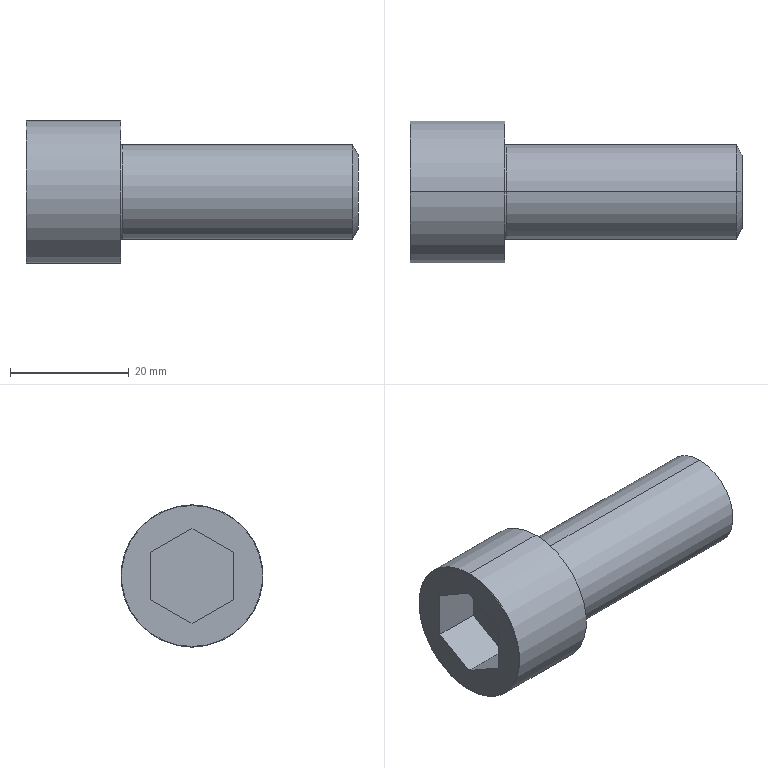Part | SolidWorks | features BlendCut 1, Cut 1, Fillet 1, LPattern 1, RevCut 1, Revolution 1 | 1 solid | 20 faces | box 56 x 24 x 24 mm | volume 13910 mm3 | plane 10 | torus 4 | cylinder 4 | cone 2 | commonest cylinder face diameters 16 x2 24 x2
STEP:
#1=CARTESIAN_POINT('',(0.,0.,11.9));
#2=VERTEX_POINT('',#1);
#3=CARTESIAN_POINT('',(0.,0.,-11.9));
#4=VERTEX_POINT('',#3);
#5=CARTESIAN_POINT('',(0.,0.,0.));
#6=DIRECTION('',(-1.,0.,0.));
#7=DIRECTION('',(0.,0.,-1.));
#8=AXIS2_PLACEMENT_3D('',#5,#6,#7);
#9=CIRCLE('',#8,11.9);
#10=EDGE_CURVE('',#2,#4,#9,.T.);
#11=ORIENTED_EDGE('',*,*,#10,.F.);
#12=CARTESIAN_POINT('',(0.1,0.,12.));
#13=VERTEX_POINT('',#12);
#14=CARTESIAN_POINT('',(0.1,0.,11.9));
#15=DIRECTION('',(0.,1.,0.));
#16=DIRECTION('',(0.,0.,1.));
#17=AXIS2_PLACEMENT_3D('',#14,#15,#16);
#18=CIRCLE('',#17,0.1);
#19=EDGE_CURVE('',#2,#13,#18,.T.);
#20=ORIENTED_EDGE('',*,*,#19,.T.);
#21=CARTESIAN_POINT('',(0.1,0.,-12.));
#22=VERTEX_POINT('',#21);
#23=CARTESIAN_POINT('',(0.1,0.,0.));
#24=DIRECTION('',(1.,0.,0.));
#25=DIRECTION('',(0.,0.,-1.));
#26=AXIS2_PLACEMENT_3D('',#23,#24,#25);
#27=CIRCLE('',#26,12.);
#28=EDGE_CURVE('',#22,#13,#27,.T.);
#29=ORIENTED_EDGE('',*,*,#28,.F.);
#30=CARTESIAN_POINT('',(0.1,0.,-11.9));
#31=DIRECTION('',(0.,-1.,0.));
#32=DIRECTION('',(0.,0.,-1.));
#33=AXIS2_PLACEMENT_3D('',#30,#31,#32);
#34=CIRCLE('',#33,0.1);
#35=EDGE_CURVE('',#4,#22,#34,.T.);
#36=ORIENTED_EDGE('',*,*,#35,.F.);
#37=EDGE_LOOP('',(#11,#20,#29,#36));
#38=FACE_OUTER_BOUND('',#37,.T.);
#39=CARTESIAN_POINT('',(0.1,0.,0.));
#40=DIRECTION('',(1.,0.,0.));
#41=DIRECTION('',(0.,0.,-1.));
#42=AXIS2_PLACEMENT_3D('',#39,#40,#41);
#43=TOROIDAL_SURFACE('',#42,11.9,0.1);
#44=ADVANCED_FACE('',(#38),#43,.T.);
#45=CARTESIAN_POINT('',(56.,0.,6.268));
#46=VERTEX_POINT('',#45);
#47=CARTESIAN_POINT('',(56.,0.,-6.268));
#48=VERTEX_POINT('',#47);
#49=CARTESIAN_POINT('',(56.,0.,0.));
#50=DIRECTION('',(-1.,0.,0.));
#51=DIRECTION('',(0.,0.,1.));
#52=AXIS2_PLACEMENT_3D('',#49,#50,#51);
#53=CIRCLE('',#52,6.268);
#54=EDGE_CURVE('',#46,#48,#53,.T.);
#55=ORIENTED_EDGE('',*,*,#54,.T.);
#56=CARTESIAN_POINT('',(55.,0.,-8.));
#57=VERTEX_POINT('',#56);
#58=CARTESIAN_POINT('',(55.,0.,-8.));
#59=DIRECTION('',(-0.5,0.,-0.866));
#60=VECTOR('',#59,1000.);
#61=LINE('',#58,#60);
#62=EDGE_CURVE('',#48,#57,#61,.T.);
#63=ORIENTED_EDGE('',*,*,#62,.T.);
#64=CARTESIAN_POINT('',(55.,0.,8.));
#65=VERTEX_POINT('',#64);
#66=CARTESIAN_POINT('',(55.,0.,0.));
#67=DIRECTION('',(-1.,0.,0.));
#68=DIRECTION('',(0.,0.,1.));
#69=AXIS2_PLACEMENT_3D('',#66,#67,#68);
#70=CIRCLE('',#69,8.);
#71=EDGE_CURVE('',#65,#57,#70,.T.);
#72=ORIENTED_EDGE('',*,*,#71,.F.);
#73=CARTESIAN_POINT('',(55.,0.,8.));
#74=DIRECTION('',(-0.5,0.,0.866));
#75=VECTOR('',#74,1000.);
#76=LINE('',#73,#75);
#77=EDGE_CURVE('',#46,#65,#76,.T.);
#78=ORIENTED_EDGE('',*,*,#77,.F.);
#79=EDGE_LOOP('',(#55,#63,#72,#78));
#80=FACE_OUTER_BOUND('',#79,.T.);
#81=CARTESIAN_POINT('',(55.,0.,0.));
#82=DIRECTION('',(-1.,0.,0.));
#83=DIRECTION('',(0.,0.,1.));
#84=AXIS2_PLACEMENT_3D('',#81,#82,#83);
#85=CONICAL_SURFACE('',#84,8.,1.047);
#86=ADVANCED_FACE('',(#80),#85,.T.);
#87=CARTESIAN_POINT('',(16.,0.,-8.2));
#88=VERTEX_POINT('',#87);
#89=CARTESIAN_POINT('',(16.,0.,8.2));
#90=VERTEX_POINT('',#89);
#91=CARTESIAN_POINT('',(16.,0.,0.));
#92=DIRECTION('',(-1.,0.,0.));
#93=DIRECTION('',(0.,0.,1.));
#94=AXIS2_PLACEMENT_3D('',#91,#92,#93);
#95=CIRCLE('',#94,8.2);
#96=EDGE_CURVE('',#88,#90,#95,.T.);
#97=ORIENTED_EDGE('',*,*,#96,.F.);
#98=CARTESIAN_POINT('',(16.2,0.,-8.));
#99=VERTEX_POINT('',#98);
#100=CARTESIAN_POINT('',(16.2,0.,-8.2));
#101=DIRECTION('',(0.,1.,0.));
#102=DIRECTION('',(0.,0.,1.));
#103=AXIS2_PLACEMENT_3D('',#100,#101,#102);
#104=CIRCLE('',#103,0.2);
#105=EDGE_CURVE('',#88,#99,#104,.T.);
#106=ORIENTED_EDGE('',*,*,#105,.T.);
#107=CARTESIAN_POINT('',(16.2,0.,8.));
#108=VERTEX_POINT('',#107);
#109=CARTESIAN_POINT('',(16.2,0.,0.));
#110=DIRECTION('',(-1.,0.,0.));
#111=DIRECTION('',(0.,0.,1.));
#112=AXIS2_PLACEMENT_3D('',#109,#110,#111);
#113=CIRCLE('',#112,8.);
#114=EDGE_CURVE('',#99,#108,#113,.T.);
#115=ORIENTED_EDGE('',*,*,#114,.T.);
#116=CARTESIAN_POINT('',(16.2,0.,8.2));
#117=DIRECTION('',(0.,-1.,0.));
#118=DIRECTION('',(0.,0.,-1.));
#119=AXIS2_PLACEMENT_3D('',#116,#117,#118);
#120=CIRCLE('',#119,0.2);
#121=EDGE_CURVE('',#90,#108,#120,.T.);
#122=ORIENTED_EDGE('',*,*,#121,.F.);
#123=EDGE_LOOP('',(#97,#106,#115,#122));
#124=FACE_OUTER_BOUND('',#123,.T.);
#125=CARTESIAN_POINT('',(16.2,0.,0.));
#126=DIRECTION('',(-1.,0.,0.));
#127=DIRECTION('',(0.,0.,1.));
#128=AXIS2_PLACEMENT_3D('',#125,#126,#127);
#129=TOROIDAL_SURFACE('',#128,8.2,0.2);
#130=ADVANCED_FACE('',(#124),#129,.F.);
#131=CARTESIAN_POINT('',(16.,0.,12.));
#132=VERTEX_POINT('',#131);
#133=CARTESIAN_POINT('',(16.,0.,-12.));
#134=VERTEX_POINT('',#133);
#135=CARTESIAN_POINT('',(16.,0.,0.));
#136=DIRECTION('',(-1.,0.,0.));
#137=DIRECTION('',(0.,0.,1.));
#138=AXIS2_PLACEMENT_3D('',#135,#136,#137);
#139=CIRCLE('',#138,12.);
#140=EDGE_CURVE('',#132,#134,#139,.T.);
#141=ORIENTED_EDGE('',*,*,#140,.T.);
#142=CARTESIAN_POINT('',(0.,0.,-12.));
#143=DIRECTION('',(-1.,0.,0.));
#144=VECTOR('',#143,1000.);
#145=LINE('',#142,#144);
#146=EDGE_CURVE('',#134,#22,#145,.T.);
#147=ORIENTED_EDGE('',*,*,#146,.T.);
#148=ORIENTED_EDGE('',*,*,#28,.T.);
#149=CARTESIAN_POINT('',(0.,0.,12.));
#150=DIRECTION('',(-1.,0.,0.));
#151=VECTOR('',#150,1000.);
#152=LINE('',#149,#151);
#153=EDGE_CURVE('',#132,#13,#152,.T.);
#154=ORIENTED_EDGE('',*,*,#153,.F.);
#155=EDGE_LOOP('',(#141,#147,#148,#154));
#156=FACE_OUTER_BOUND('',#155,.T.);
#157=CARTESIAN_POINT('',(0.,0.,0.));
#158=DIRECTION('',(-1.,0.,0.));
#159=DIRECTION('',(0.,0.,1.));
#160=AXIS2_PLACEMENT_3D('',#157,#158,#159);
#161=CYLINDRICAL_SURFACE('',#160,12.);
#162=ADVANCED_FACE('',(#156),#161,.T.);
#163=ORIENTED_EDGE('',*,*,#71,.T.);
#164=CARTESIAN_POINT('',(0.,0.,-8.));
#165=DIRECTION('',(-1.,0.,0.));
#166=VECTOR('',#165,1000.);
#167=LINE('',#164,#166);
#168=EDGE_CURVE('',#57,#99,#167,.T.);
#169=ORIENTED_EDGE('',*,*,#168,.T.);
#170=CARTESIAN_POINT('',(16.2,0.,0.));
#171=DIRECTION('',(-1.,0.,0.));
#172=DIRECTION('',(0.,0.,1.));
#173=AXIS2_PLACEMENT_3D('',#170,#171,#172);
#174=CIRCLE('',#173,8.);
#175=EDGE_CURVE('',#108,#99,#174,.T.);
#176=ORIENTED_EDGE('',*,*,#175,.F.);
#177=CARTESIAN_POINT('',(0.,0.,8.));
#178=DIRECTION('',(-1.,0.,0.));
#179=VECTOR('',#178,1000.);
#180=LINE('',#177,#179);
#181=EDGE_CURVE('',#65,#108,#180,.T.);
#182=ORIENTED_EDGE('',*,*,#181,.F.);
#183=EDGE_LOOP('',(#163,#169,#176,#182));
#184=FACE_OUTER_BOUND('',#183,.T.);
#185=CARTESIAN_POINT('',(0.,0.,0.));
#186=DIRECTION('',(-1.,0.,0.));
#187=DIRECTION('',(0.,0.,1.));
#188=AXIS2_PLACEMENT_3D('',#185,#186,#187);
#189=CYLINDRICAL_SURFACE('',#188,8.);
#190=ADVANCED_FACE('',(#184),#189,.T.);
#191=ORIENTED_EDGE('',*,*,#168,.F.);
#192=CARTESIAN_POINT('',(55.,0.,0.));
#193=DIRECTION('',(-1.,0.,0.));
#194=DIRECTION('',(0.,0.,1.));
#195=AXIS2_PLACEMENT_3D('',#192,#193,#194);
#196=CIRCLE('',#195,8.);
#197=EDGE_CURVE('',#57,#65,#196,.T.);
#198=ORIENTED_EDGE('',*,*,#197,.T.);
#199=ORIENTED_EDGE('',*,*,#181,.T.);
#200=ORIENTED_EDGE('',*,*,#114,.F.);
#201=EDGE_LOOP('',(#191,#198,#199,#200));
#202=FACE_OUTER_BOUND('',#201,.T.);
#203=CARTESIAN_POINT('',(0.,0.,0.));
#204=DIRECTION('',(-1.,0.,0.));
#205=DIRECTION('',(0.,0.,1.));
#206=AXIS2_PLACEMENT_3D('',#203,#204,#205);
#207=CYLINDRICAL_SURFACE('',#206,8.);
#208=ADVANCED_FACE('',(#202),#207,.T.);
#209=CARTESIAN_POINT('',(0.,0.,0.));
#210=DIRECTION('',(-1.,0.,0.));
#211=DIRECTION('',(0.,0.,-1.));
#212=AXIS2_PLACEMENT_3D('',#209,#210,#211);
#213=CIRCLE('',#212,11.9);
#214=EDGE_CURVE('',#4,#2,#213,.T.);
#215=ORIENTED_EDGE('',*,*,#214,.T.);
#216=ORIENTED_EDGE('',*,*,#10,.T.);
#217=EDGE_LOOP('',(#215,#216));
#218=FACE_OUTER_BOUND('',#217,.T.);
#219=CARTESIAN_POINT('',(0.,0.,8.));
#220=VERTEX_POINT('',#219);
#221=CARTESIAN_POINT('',(0.,6.928,4.));
#222=VERTEX_POINT('',#221);
#223=CARTESIAN_POINT('',(0.,0.,8.));
#224=DIRECTION('',(0.,0.866,-0.5));
#225=VECTOR('',#224,1000.);
#226=LINE('',#223,#225);
#227=EDGE_CURVE('',#220,#222,#226,.T.);
#228=ORIENTED_EDGE('',*,*,#227,.F.);
#229=CARTESIAN_POINT('',(0.,-6.928,4.));
#230=VERTEX_POINT('',#229);
#231=CARTESIAN_POINT('',(0.,-6.928,4.));
#232=DIRECTION('',(0.,0.866,0.5));
#233=VECTOR('',#232,1000.);
#234=LINE('',#231,#233);
#235=EDGE_CURVE('',#230,#220,#234,.T.);
#236=ORIENTED_EDGE('',*,*,#235,.F.);
#237=CARTESIAN_POINT('',(0.,-6.928,-4.));
#238=VERTEX_POINT('',#237);
#239=CARTESIAN_POINT('',(0.,-6.928,-4.));
#240=DIRECTION('',(0.,0.,1.));
#241=VECTOR('',#240,1000.);
#242=LINE('',#239,#241);
#243=EDGE_CURVE('',#238,#230,#242,.T.);
#244=ORIENTED_EDGE('',*,*,#243,.F.);
#245=CARTESIAN_POINT('',(0.,0.,-8.));
#246=VERTEX_POINT('',#245);
#247=CARTESIAN_POINT('',(0.,0.,-8.));
#248=DIRECTION('',(0.,-0.866,0.5));
#249=VECTOR('',#248,1000.);
#250=LINE('',#247,#249);
#251=EDGE_CURVE('',#246,#238,#250,.T.);
#252=ORIENTED_EDGE('',*,*,#251,.F.);
#253=CARTESIAN_POINT('',(0.,6.928,-4.));
#254=VERTEX_POINT('',#253);
#255=CARTESIAN_POINT('',(0.,6.928,-4.));
#256=DIRECTION('',(0.,-0.866,-0.5));
#257=VECTOR('',#256,1000.);
#258=LINE('',#255,#257);
#259=EDGE_CURVE('',#254,#246,#258,.T.);
#260=ORIENTED_EDGE('',*,*,#259,.F.);
#261=CARTESIAN_POINT('',(0.,6.928,4.));
#262=DIRECTION('',(0.,0.,-1.));
#263=VECTOR('',#262,1000.);
#264=LINE('',#261,#263);
#265=EDGE_CURVE('',#222,#254,#264,.T.);
#266=ORIENTED_EDGE('',*,*,#265,.F.);
#267=EDGE_LOOP('',(#228,#236,#244,#252,#260,#266));
#268=FACE_BOUND('',#267,.T.);
#269=CARTESIAN_POINT('',(0.,0.,0.));
#270=DIRECTION('',(1.,0.,0.));
#271=DIRECTION('',(0.,0.,-1.));
#272=AXIS2_PLACEMENT_3D('',#269,#270,#271);
#273=PLANE('',#272);
#274=ADVANCED_FACE('',(#218,#268),#273,.F.);
#275=ORIENTED_EDGE('',*,*,#146,.F.);
#276=CARTESIAN_POINT('',(16.,0.,0.));
#277=DIRECTION('',(-1.,0.,0.));
#278=DIRECTION('',(0.,0.,1.));
#279=AXIS2_PLACEMENT_3D('',#276,#277,#278);
#280=CIRCLE('',#279,12.);
#281=EDGE_CURVE('',#134,#132,#280,.T.);
#282=ORIENTED_EDGE('',*,*,#281,.T.);
#283=ORIENTED_EDGE('',*,*,#153,.T.);
#284=CARTESIAN_POINT('',(0.1,0.,0.));
#285=DIRECTION('',(1.,0.,0.));
#286=DIRECTION('',(0.,0.,-1.));
#287=AXIS2_PLACEMENT_3D('',#284,#285,#286);
#288=CIRCLE('',#287,12.);
#289=EDGE_CURVE('',#13,#22,#288,.T.);
#290=ORIENTED_EDGE('',*,*,#289,.T.);
#291=EDGE_LOOP('',(#275,#282,#283,#290));
#292=FACE_OUTER_BOUND('',#291,.T.);
#293=CARTESIAN_POINT('',(0.,0.,0.));
#294=DIRECTION('',(-1.,0.,0.));
#295=DIRECTION('',(0.,0.,1.));
#296=AXIS2_PLACEMENT_3D('',#293,#294,#295);
#297=CYLINDRICAL_SURFACE('',#296,12.);
#298=ADVANCED_FACE('',(#292),#297,.T.);
#299=ORIENTED_EDGE('',*,*,#140,.F.);
#300=ORIENTED_EDGE('',*,*,#281,.F.);
#301=EDGE_LOOP('',(#299,#300));
#302=FACE_OUTER_BOUND('',#301,.T.);
#303=CARTESIAN_POINT('',(16.,0.,0.));
#304=DIRECTION('',(-1.,0.,0.));
#305=DIRECTION('',(0.,0.,1.));
#306=AXIS2_PLACEMENT_3D('',#303,#304,#305);
#307=CIRCLE('',#306,8.2);
#308=EDGE_CURVE('',#90,#88,#307,.T.);
#309=ORIENTED_EDGE('',*,*,#308,.T.);
#310=ORIENTED_EDGE('',*,*,#96,.T.);
#311=EDGE_LOOP('',(#309,#310));
#312=FACE_BOUND('',#311,.T.);
#313=CARTESIAN_POINT('',(16.,12.,0.));
#314=DIRECTION('',(-1.,0.,0.));
#315=DIRECTION('',(0.,0.,1.));
#316=AXIS2_PLACEMENT_3D('',#313,#314,#315);
#317=PLANE('',#316);
#318=ADVANCED_FACE('',(#302,#312),#317,.F.);
#319=ORIENTED_EDGE('',*,*,#105,.F.);
#320=ORIENTED_EDGE('',*,*,#308,.F.);
#321=ORIENTED_EDGE('',*,*,#121,.T.);
#322=ORIENTED_EDGE('',*,*,#175,.T.);
#323=EDGE_LOOP('',(#319,#320,#321,#322));
#324=FACE_OUTER_BOUND('',#323,.T.);
#325=CARTESIAN_POINT('',(16.2,0.,0.));
#326=DIRECTION('',(-1.,0.,0.));
#327=DIRECTION('',(0.,0.,1.));
#328=AXIS2_PLACEMENT_3D('',#325,#326,#327);
#329=TOROIDAL_SURFACE('',#328,8.2,0.2);
#330=ADVANCED_FACE('',(#324),#329,.F.);
#331=ORIENTED_EDGE('',*,*,#235,.T.);
#332=CARTESIAN_POINT('',(8.,0.,8.));
#333=VERTEX_POINT('',#332);
#334=CARTESIAN_POINT('',(8.,0.,8.));
#335=DIRECTION('',(-1.,0.,0.));
#336=VECTOR('',#335,1000.);
#337=LINE('',#334,#336);
#338=EDGE_CURVE('',#333,#220,#337,.T.);
#339=ORIENTED_EDGE('',*,*,#338,.F.);
#340=CARTESIAN_POINT('',(8.,-6.928,4.));
#341=VERTEX_POINT('',#340);
#342=CARTESIAN_POINT('',(8.,-6.928,4.));
#343=DIRECTION('',(0.,0.866,0.5));
#344=VECTOR('',#343,1000.);
#345=LINE('',#342,#344);
#346=EDGE_CURVE('',#341,#333,#345,.T.);
#347=ORIENTED_EDGE('',*,*,#346,.F.);
#348=CARTESIAN_POINT('',(8.,-6.928,4.));
#349=DIRECTION('',(-1.,0.,0.));
#350=VECTOR('',#349,1000.);
#351=LINE('',#348,#350);
#352=EDGE_CURVE('',#341,#230,#351,.T.);
#353=ORIENTED_EDGE('',*,*,#352,.T.);
#354=EDGE_LOOP('',(#331,#339,#347,#353));
#355=FACE_OUTER_BOUND('',#354,.T.);
#356=CARTESIAN_POINT('',(8.,-6.928,4.));
#357=DIRECTION('',(0.,-0.5,0.866));
#358=DIRECTION('',(0.,-0.866,-0.5));
#359=AXIS2_PLACEMENT_3D('',#356,#357,#358);
#360=PLANE('',#359);
#361=ADVANCED_FACE('',(#355),#360,.F.);
#362=ORIENTED_EDGE('',*,*,#243,.T.);
#363=ORIENTED_EDGE('',*,*,#352,.F.);
#364=CARTESIAN_POINT('',(8.,-6.928,-4.));
#365=VERTEX_POINT('',#364);
#366=CARTESIAN_POINT('',(8.,-6.928,-4.));
#367=DIRECTION('',(0.,0.,1.));
#368=VECTOR('',#367,1000.);
#369=LINE('',#366,#368);
#370=EDGE_CURVE('',#365,#341,#369,.T.);
#371=ORIENTED_EDGE('',*,*,#370,.F.);
#372=CARTESIAN_POINT('',(8.,-6.928,-4.));
#373=DIRECTION('',(-1.,0.,0.));
#374=VECTOR('',#373,1000.);
#375=LINE('',#372,#374);
#376=EDGE_CURVE('',#365,#238,#375,.T.);
#377=ORIENTED_EDGE('',*,*,#376,.T.);
#378=EDGE_LOOP('',(#362,#363,#371,#377));
#379=FACE_OUTER_BOUND('',#378,.T.);
#380=CARTESIAN_POINT('',(8.,-6.928,-4.));
#381=DIRECTION('',(0.,-1.,0.));
#382=DIRECTION('',(0.,0.,-1.));
#383=AXIS2_PLACEMENT_3D('',#380,#381,#382);
#384=PLANE('',#383);
#385=ADVANCED_FACE('',(#379),#384,.F.);
#386=ORIENTED_EDGE('',*,*,#251,.T.);
#387=ORIENTED_EDGE('',*,*,#376,.F.);
#388=CARTESIAN_POINT('',(8.,0.,-8.));
#389=VERTEX_POINT('',#388);
#390=CARTESIAN_POINT('',(8.,0.,-8.));
#391=DIRECTION('',(0.,-0.866,0.5));
#392=VECTOR('',#391,1000.);
#393=LINE('',#390,#392);
#394=EDGE_CURVE('',#389,#365,#393,.T.);
#395=ORIENTED_EDGE('',*,*,#394,.F.);
#396=CARTESIAN_POINT('',(8.,0.,-8.));
#397=DIRECTION('',(-1.,0.,0.));
#398=VECTOR('',#397,1000.);
#399=LINE('',#396,#398);
#400=EDGE_CURVE('',#389,#246,#399,.T.);
#401=ORIENTED_EDGE('',*,*,#400,.T.);
#402=EDGE_LOOP('',(#386,#387,#395,#401));
#403=FACE_OUTER_BOUND('',#402,.T.);
#404=CARTESIAN_POINT('',(8.,0.,-8.));
#405=DIRECTION('',(0.,-0.5,-0.866));
#406=DIRECTION('',(0.,0.866,-0.5));
#407=AXIS2_PLACEMENT_3D('',#404,#405,#406);
#408=PLANE('',#407);
#409=ADVANCED_FACE('',(#403),#408,.F.);
#410=ORIENTED_EDGE('',*,*,#259,.T.);
#411=ORIENTED_EDGE('',*,*,#400,.F.);
#412=CARTESIAN_POINT('',(8.,6.928,-4.));
#413=VERTEX_POINT('',#412);
#414=CARTESIAN_POINT('',(8.,6.928,-4.));
#415=DIRECTION('',(0.,-0.866,-0.5));
#416=VECTOR('',#415,1000.);
#417=LINE('',#414,#416);
#418=EDGE_CURVE('',#413,#389,#417,.T.);
#419=ORIENTED_EDGE('',*,*,#418,.F.);
#420=CARTESIAN_POINT('',(8.,6.928,-4.));
#421=DIRECTION('',(-1.,0.,0.));
#422=VECTOR('',#421,1000.);
#423=LINE('',#420,#422);
#424=EDGE_CURVE('',#413,#254,#423,.T.);
#425=ORIENTED_EDGE('',*,*,#424,.T.);
#426=EDGE_LOOP('',(#410,#411,#419,#425));
#427=FACE_OUTER_BOUND('',#426,.T.);
#428=CARTESIAN_POINT('',(8.,6.928,-4.));
#429=DIRECTION('',(0.,0.5,-0.866));
#430=DIRECTION('',(0.,0.866,0.5));
#431=AXIS2_PLACEMENT_3D('',#428,#429,#430);
#432=PLANE('',#431);
#433=ADVANCED_FACE('',(#427),#432,.F.);
#434=ORIENTED_EDGE('',*,*,#265,.T.);
#435=ORIENTED_EDGE('',*,*,#424,.F.);
#436=CARTESIAN_POINT('',(8.,6.928,4.));
#437=VERTEX_POINT('',#436);
#438=CARTESIAN_POINT('',(8.,6.928,4.));
#439=DIRECTION('',(0.,0.,-1.));
#440=VECTOR('',#439,1000.);
#441=LINE('',#438,#440);
#442=EDGE_CURVE('',#437,#413,#441,.T.);
#443=ORIENTED_EDGE('',*,*,#442,.F.);
#444=CARTESIAN_POINT('',(8.,6.928,4.));
#445=DIRECTION('',(-1.,0.,0.));
#446=VECTOR('',#445,1000.);
#447=LINE('',#444,#446);
#448=EDGE_CURVE('',#437,#222,#447,.T.);
#449=ORIENTED_EDGE('',*,*,#448,.T.);
#450=EDGE_LOOP('',(#434,#435,#443,#449));
#451=FACE_OUTER_BOUND('',#450,.T.);
#452=CARTESIAN_POINT('',(8.,6.928,4.));
#453=DIRECTION('',(0.,1.,0.));
#454=DIRECTION('',(0.,0.,1.));
#455=AXIS2_PLACEMENT_3D('',#452,#453,#454);
#456=PLANE('',#455);
#457=ADVANCED_FACE('',(#451),#456,.F.);
#458=ORIENTED_EDGE('',*,*,#227,.T.);
#459=ORIENTED_EDGE('',*,*,#448,.F.);
#460=CARTESIAN_POINT('',(8.,0.,8.));
#461=DIRECTION('',(0.,0.866,-0.5));
#462=VECTOR('',#461,1000.);
#463=LINE('',#460,#462);
#464=EDGE_CURVE('',#333,#437,#463,.T.);
#465=ORIENTED_EDGE('',*,*,#464,.F.);
#466=ORIENTED_EDGE('',*,*,#338,.T.);
#467=EDGE_LOOP('',(#458,#459,#465,#466));
#468=FACE_OUTER_BOUND('',#467,.T.);
#469=CARTESIAN_POINT('',(8.,0.,8.));
#470=DIRECTION('',(0.,0.5,0.866));
#471=DIRECTION('',(0.,-0.866,0.5));
#472=AXIS2_PLACEMENT_3D('',#469,#470,#471);
#473=PLANE('',#472);
#474=ADVANCED_FACE('',(#468),#473,.F.);
#475=ORIENTED_EDGE('',*,*,#346,.T.);
#476=ORIENTED_EDGE('',*,*,#464,.T.);
#477=ORIENTED_EDGE('',*,*,#442,.T.);
#478=ORIENTED_EDGE('',*,*,#418,.T.);
#479=ORIENTED_EDGE('',*,*,#394,.T.);
#480=ORIENTED_EDGE('',*,*,#370,.T.);
#481=EDGE_LOOP('',(#475,#476,#477,#478,#479,#480));
#482=FACE_OUTER_BOUND('',#481,.T.);
#483=CARTESIAN_POINT('',(8.,-6.928,4.));
#484=DIRECTION('',(1.,0.,0.));
#485=DIRECTION('',(0.,0.,-1.));
#486=AXIS2_PLACEMENT_3D('',#483,#484,#485);
#487=PLANE('',#486);
#488=ADVANCED_FACE('',(#482),#487,.F.);
#489=ORIENTED_EDGE('',*,*,#62,.F.);
#490=CARTESIAN_POINT('',(56.,0.,0.));
#491=DIRECTION('',(-1.,0.,0.));
#492=DIRECTION('',(0.,0.,1.));
#493=AXIS2_PLACEMENT_3D('',#490,#491,#492);
#494=CIRCLE('',#493,6.268);
#495=EDGE_CURVE('',#48,#46,#494,.T.);
#496=ORIENTED_EDGE('',*,*,#495,.T.);
#497=ORIENTED_EDGE('',*,*,#77,.T.);
#498=ORIENTED_EDGE('',*,*,#197,.F.);
#499=EDGE_LOOP('',(#489,#496,#497,#498));
#500=FACE_OUTER_BOUND('',#499,.T.);
#501=CARTESIAN_POINT('',(55.,0.,0.));
#502=DIRECTION('',(-1.,0.,0.));
#503=DIRECTION('',(0.,0.,1.));
#504=AXIS2_PLACEMENT_3D('',#501,#502,#503);
#505=CONICAL_SURFACE('',#504,8.,1.047);
#506=ADVANCED_FACE('',(#500),#505,.T.);
#507=ORIENTED_EDGE('',*,*,#54,.F.);
#508=ORIENTED_EDGE('',*,*,#495,.F.);
#509=EDGE_LOOP('',(#507,#508));
#510=FACE_OUTER_BOUND('',#509,.T.);
#511=CARTESIAN_POINT('',(56.,8.,0.));
#512=DIRECTION('',(-1.,0.,0.));
#513=DIRECTION('',(0.,0.,1.));
#514=AXIS2_PLACEMENT_3D('',#511,#512,#513);
#515=PLANE('',#514);
#516=ADVANCED_FACE('',(#510),#515,.F.);
#517=ORIENTED_EDGE('',*,*,#19,.F.);
#518=ORIENTED_EDGE('',*,*,#214,.F.);
#519=ORIENTED_EDGE('',*,*,#35,.T.);
#520=ORIENTED_EDGE('',*,*,#289,.F.);
#521=EDGE_LOOP('',(#517,#518,#519,#520));
#522=FACE_OUTER_BOUND('',#521,.T.);
#523=CARTESIAN_POINT('',(0.1,0.,0.));
#524=DIRECTION('',(1.,0.,0.));
#525=DIRECTION('',(0.,0.,-1.));
#526=AXIS2_PLACEMENT_3D('',#523,#524,#525);
#527=TOROIDAL_SURFACE('',#526,11.9,0.1);
#528=ADVANCED_FACE('',(#522),#527,.T.);
#529=CLOSED_SHELL('',(#44,#86,#130,#162,#190,#208,#274,#298,#318,#330,#361,#385,#409,#433,#457,#474,#488,#506,#516,#528));
#530=MANIFOLD_SOLID_BREP('',#529);
#531=CARTESIAN_POINT('',(0.,0.,0.));
#532=DIRECTION('',(0.,0.,1.));
#533=DIRECTION('',(1.,0.,0.));
#534=AXIS2_PLACEMENT_3D('',#531,#532,#533);
#535=(LENGTH_UNIT()NAMED_UNIT(*)SI_UNIT(.MILLI.,.METRE.));
#536=UNCERTAINTY_MEASURE_WITH_UNIT(LENGTH_MEASURE(0.00001),#535,'','');
#537=(NAMED_UNIT(*)PLANE_ANGLE_UNIT()SI_UNIT($,.RADIAN.));
#538=(NAMED_UNIT(*)SI_UNIT($,.STERADIAN.)SOLID_ANGLE_UNIT());
#539=(GEOMETRIC_REPRESENTATION_CONTEXT(3)GLOBAL_UNCERTAINTY_ASSIGNED_CONTEXT((#536))GLOBAL_UNIT_ASSIGNED_CONTEXT((#535,#537,#538))REPRESENTATION_CONTEXT('',''));
#540=ADVANCED_BREP_SHAPE_REPRESENTATION('',(#530,#534),#539);